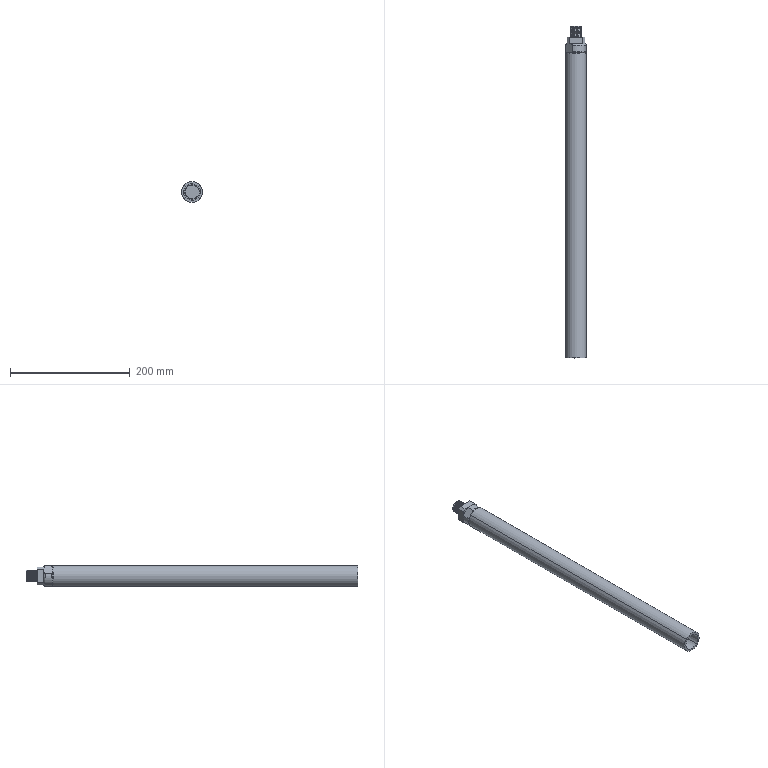Part | STEP file | 60-400mm push rod | 3 solids | 96 faces | box 35 x 555 x 35 mm | volume 228632 mm3 | cylinder 57 | plane 23 | torus 8 | spline 8 | commonest cylinder face diameters 20 x32 25 x18 34 x3 28 x2 35 x2